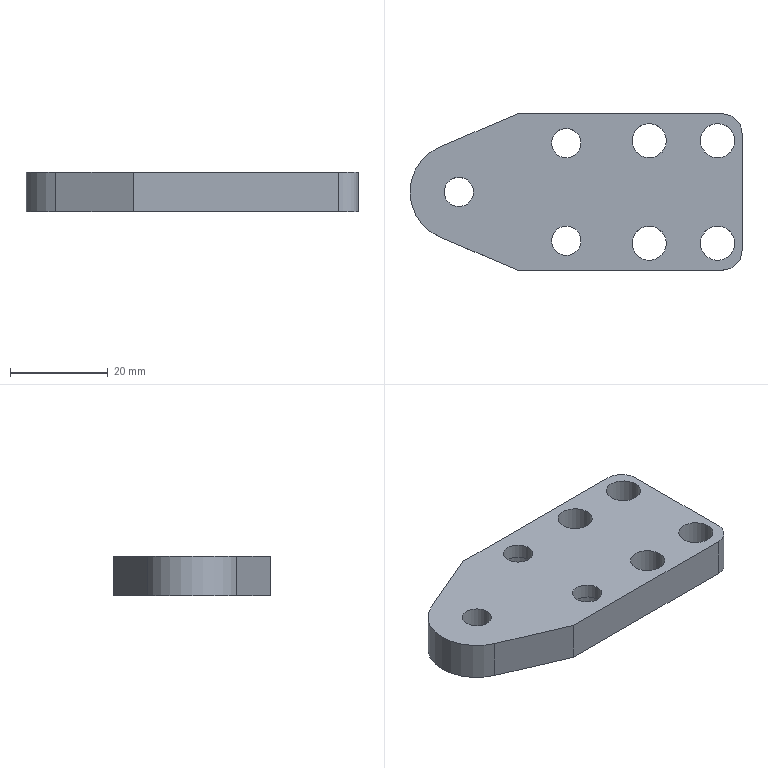Part | NX | features BREP 1, DATUM_CSYS 1 | 1 solid | 21 faces | box 68 x 32 x 8 mm | volume 13164 mm3 | cylinder 12 | plane 9 | commonest cylinder face diameters 7 x4 6 x3 8 x2 10 x2 20 x1
STEP:
#1=CARTESIAN_POINT('',(-34.,16.,0.));
#2=VERTEX_POINT('',#1);
#3=CARTESIAN_POINT('',(-49.928,9.196,0.));
#4=VERTEX_POINT('',#3);
#5=CARTESIAN_POINT('',(-34.,16.,0.));
#6=DIRECTION('',(-0.9196,-0.3928,0.));
#7=VECTOR('',#6,1000.);
#8=LINE('',#5,#7);
#9=EDGE_CURVE('',#2,#4,#8,.T.);
#10=ORIENTED_EDGE('',*,*,#9,.T.);
#11=CARTESIAN_POINT('',(-49.928,9.196,8.));
#12=VERTEX_POINT('',#11);
#13=CARTESIAN_POINT('',(-49.928,9.196,0.));
#14=DIRECTION('',(0.,0.,1.));
#15=VECTOR('',#14,1000.);
#16=LINE('',#13,#15);
#17=EDGE_CURVE('',#4,#12,#16,.T.);
#18=ORIENTED_EDGE('',*,*,#17,.T.);
#19=CARTESIAN_POINT('',(-34.,16.,8.));
#20=VERTEX_POINT('',#19);
#21=CARTESIAN_POINT('',(-34.,16.,8.));
#22=DIRECTION('',(-0.9196,-0.3928,0.));
#23=VECTOR('',#22,1000.);
#24=LINE('',#21,#23);
#25=EDGE_CURVE('',#20,#12,#24,.T.);
#26=ORIENTED_EDGE('',*,*,#25,.F.);
#27=CARTESIAN_POINT('',(-34.,16.,0.));
#28=DIRECTION('',(0.,0.,1.));
#29=VECTOR('',#28,1000.);
#30=LINE('',#27,#29);
#31=EDGE_CURVE('',#2,#20,#30,.T.);
#32=ORIENTED_EDGE('',*,*,#31,.F.);
#33=EDGE_LOOP('',(#10,#18,#26,#32));
#34=FACE_BOUND('',#33,.T.);
#35=CARTESIAN_POINT('',(-41.964,12.598,4.));
#36=DIRECTION('',(-0.3928,0.9196,0.));
#37=DIRECTION('',(0.9196,0.3928,0.));
#38=AXIS2_PLACEMENT_3D('',#35,#36,#37);
#39=PLANE('',#38);
#40=ADVANCED_FACE('',(#34),#39,.T.);
#41=CARTESIAN_POINT('',(-49.928,-9.196,0.));
#42=VERTEX_POINT('',#41);
#43=CARTESIAN_POINT('',(-46.,0.,0.));
#44=DIRECTION('',(0.,0.,1.));
#45=DIRECTION('',(-0.3928,0.9196,0.));
#46=AXIS2_PLACEMENT_3D('',#43,#44,#45);
#47=CIRCLE('',#46,10.);
#48=EDGE_CURVE('',#4,#42,#47,.T.);
#49=ORIENTED_EDGE('',*,*,#48,.T.);
#50=CARTESIAN_POINT('',(-49.928,-9.196,8.));
#51=VERTEX_POINT('',#50);
#52=CARTESIAN_POINT('',(-49.928,-9.196,0.));
#53=DIRECTION('',(0.,0.,1.));
#54=VECTOR('',#53,1000.);
#55=LINE('',#52,#54);
#56=EDGE_CURVE('',#42,#51,#55,.T.);
#57=ORIENTED_EDGE('',*,*,#56,.T.);
#58=CARTESIAN_POINT('',(-46.,0.,8.));
#59=DIRECTION('',(0.,0.,1.));
#60=DIRECTION('',(-0.3928,0.9196,0.));
#61=AXIS2_PLACEMENT_3D('',#58,#59,#60);
#62=CIRCLE('',#61,10.);
#63=EDGE_CURVE('',#12,#51,#62,.T.);
#64=ORIENTED_EDGE('',*,*,#63,.F.);
#65=ORIENTED_EDGE('',*,*,#17,.F.);
#66=EDGE_LOOP('',(#49,#57,#64,#65));
#67=FACE_BOUND('',#66,.T.);
#68=CARTESIAN_POINT('',(-46.,0.,0.));
#69=DIRECTION('',(0.,0.,1.));
#70=DIRECTION('',(0.3928,-0.9196,0.));
#71=AXIS2_PLACEMENT_3D('',#68,#69,#70);
#72=CYLINDRICAL_SURFACE('',#71,10.);
#73=ADVANCED_FACE('',(#67),#72,.T.);
#74=CARTESIAN_POINT('',(-34.,-16.,0.));
#75=VERTEX_POINT('',#74);
#76=CARTESIAN_POINT('',(-49.928,-9.196,0.));
#77=DIRECTION('',(0.9196,-0.3928,0.));
#78=VECTOR('',#77,1000.);
#79=LINE('',#76,#78);
#80=EDGE_CURVE('',#42,#75,#79,.T.);
#81=ORIENTED_EDGE('',*,*,#80,.T.);
#82=CARTESIAN_POINT('',(-34.,-16.,8.));
#83=VERTEX_POINT('',#82);
#84=CARTESIAN_POINT('',(-34.,-16.,0.));
#85=DIRECTION('',(0.,0.,1.));
#86=VECTOR('',#85,1000.);
#87=LINE('',#84,#86);
#88=EDGE_CURVE('',#75,#83,#87,.T.);
#89=ORIENTED_EDGE('',*,*,#88,.T.);
#90=CARTESIAN_POINT('',(-49.928,-9.196,8.));
#91=DIRECTION('',(0.9196,-0.3928,0.));
#92=VECTOR('',#91,1000.);
#93=LINE('',#90,#92);
#94=EDGE_CURVE('',#51,#83,#93,.T.);
#95=ORIENTED_EDGE('',*,*,#94,.F.);
#96=ORIENTED_EDGE('',*,*,#56,.F.);
#97=EDGE_LOOP('',(#81,#89,#95,#96));
#98=FACE_BOUND('',#97,.T.);
#99=CARTESIAN_POINT('',(-41.964,-12.598,4.));
#100=DIRECTION('',(-0.3928,-0.9196,0.));
#101=DIRECTION('',(-0.9196,0.3928,0.));
#102=AXIS2_PLACEMENT_3D('',#99,#100,#101);
#103=PLANE('',#102);
#104=ADVANCED_FACE('',(#98),#103,.T.);
#105=CARTESIAN_POINT('',(12.,-12.,0.));
#106=VERTEX_POINT('',#105);
#107=CARTESIAN_POINT('',(12.,12.,0.));
#108=VERTEX_POINT('',#107);
#109=CARTESIAN_POINT('',(12.,-12.,0.));
#110=DIRECTION('',(0.,1.,0.));
#111=VECTOR('',#110,1000.);
#112=LINE('',#109,#111);
#113=EDGE_CURVE('',#106,#108,#112,.T.);
#114=ORIENTED_EDGE('',*,*,#113,.T.);
#115=CARTESIAN_POINT('',(12.,12.,8.));
#116=VERTEX_POINT('',#115);
#117=CARTESIAN_POINT('',(12.,12.,0.));
#118=DIRECTION('',(0.,0.,1.));
#119=VECTOR('',#118,1000.);
#120=LINE('',#117,#119);
#121=EDGE_CURVE('',#108,#116,#120,.T.);
#122=ORIENTED_EDGE('',*,*,#121,.T.);
#123=CARTESIAN_POINT('',(12.,-12.,8.));
#124=VERTEX_POINT('',#123);
#125=CARTESIAN_POINT('',(12.,-12.,8.));
#126=DIRECTION('',(0.,1.,0.));
#127=VECTOR('',#126,1000.);
#128=LINE('',#125,#127);
#129=EDGE_CURVE('',#124,#116,#128,.T.);
#130=ORIENTED_EDGE('',*,*,#129,.F.);
#131=CARTESIAN_POINT('',(12.,-12.,0.));
#132=DIRECTION('',(0.,0.,1.));
#133=VECTOR('',#132,1000.);
#134=LINE('',#131,#133);
#135=EDGE_CURVE('',#106,#124,#134,.T.);
#136=ORIENTED_EDGE('',*,*,#135,.F.);
#137=EDGE_LOOP('',(#114,#122,#130,#136));
#138=FACE_BOUND('',#137,.T.);
#139=CARTESIAN_POINT('',(12.,0.,4.));
#140=DIRECTION('',(1.,0.,0.));
#141=DIRECTION('',(0.,-1.,0.));
#142=AXIS2_PLACEMENT_3D('',#139,#140,#141);
#143=PLANE('',#142);
#144=ADVANCED_FACE('',(#138),#143,.T.);
#145=CARTESIAN_POINT('',(8.,16.,8.));
#146=VERTEX_POINT('',#145);
#147=CARTESIAN_POINT('',(8.,16.,8.));
#148=DIRECTION('',(-1.,0.,0.));
#149=VECTOR('',#148,1000.);
#150=LINE('',#147,#149);
#151=EDGE_CURVE('',#146,#20,#150,.T.);
#152=ORIENTED_EDGE('',*,*,#151,.F.);
#153=CARTESIAN_POINT('',(8.,16.,0.));
#154=VERTEX_POINT('',#153);
#155=CARTESIAN_POINT('',(8.,16.,0.));
#156=DIRECTION('',(0.,0.,1.));
#157=VECTOR('',#156,1000.);
#158=LINE('',#155,#157);
#159=EDGE_CURVE('',#154,#146,#158,.T.);
#160=ORIENTED_EDGE('',*,*,#159,.F.);
#161=CARTESIAN_POINT('',(8.,16.,0.));
#162=DIRECTION('',(-1.,0.,0.));
#163=VECTOR('',#162,1000.);
#164=LINE('',#161,#163);
#165=EDGE_CURVE('',#154,#2,#164,.T.);
#166=ORIENTED_EDGE('',*,*,#165,.T.);
#167=ORIENTED_EDGE('',*,*,#31,.T.);
#168=EDGE_LOOP('',(#152,#160,#166,#167));
#169=FACE_BOUND('',#168,.T.);
#170=CARTESIAN_POINT('',(-11.,16.,4.));
#171=DIRECTION('',(0.,1.,0.));
#172=DIRECTION('',(1.,0.,0.));
#173=AXIS2_PLACEMENT_3D('',#170,#171,#172);
#174=PLANE('',#173);
#175=ADVANCED_FACE('',(#169),#174,.T.);
#176=CARTESIAN_POINT('',(8.,-16.,0.));
#177=VERTEX_POINT('',#176);
#178=CARTESIAN_POINT('',(-34.,-16.,0.));
#179=DIRECTION('',(1.,0.,0.));
#180=VECTOR('',#179,1000.);
#181=LINE('',#178,#180);
#182=EDGE_CURVE('',#75,#177,#181,.T.);
#183=ORIENTED_EDGE('',*,*,#182,.T.);
#184=CARTESIAN_POINT('',(8.,-16.,8.));
#185=VERTEX_POINT('',#184);
#186=CARTESIAN_POINT('',(8.,-16.,0.));
#187=DIRECTION('',(0.,0.,1.));
#188=VECTOR('',#187,1000.);
#189=LINE('',#186,#188);
#190=EDGE_CURVE('',#177,#185,#189,.T.);
#191=ORIENTED_EDGE('',*,*,#190,.T.);
#192=CARTESIAN_POINT('',(-34.,-16.,8.));
#193=DIRECTION('',(1.,0.,0.));
#194=VECTOR('',#193,1000.);
#195=LINE('',#192,#194);
#196=EDGE_CURVE('',#83,#185,#195,.T.);
#197=ORIENTED_EDGE('',*,*,#196,.F.);
#198=ORIENTED_EDGE('',*,*,#88,.F.);
#199=EDGE_LOOP('',(#183,#191,#197,#198));
#200=FACE_BOUND('',#199,.T.);
#201=CARTESIAN_POINT('',(-11.,-16.,4.));
#202=DIRECTION('',(0.,-1.,0.));
#203=DIRECTION('',(-1.,0.,0.));
#204=AXIS2_PLACEMENT_3D('',#201,#202,#203);
#205=PLANE('',#204);
#206=ADVANCED_FACE('',(#200),#205,.T.);
#207=CARTESIAN_POINT('',(8.,-12.,0.));
#208=DIRECTION('',(0.,0.,1.));
#209=DIRECTION('',(0.,-1.,0.));
#210=AXIS2_PLACEMENT_3D('',#207,#208,#209);
#211=CIRCLE('',#210,4.);
#212=EDGE_CURVE('',#177,#106,#211,.T.);
#213=ORIENTED_EDGE('',*,*,#212,.T.);
#214=ORIENTED_EDGE('',*,*,#135,.T.);
#215=CARTESIAN_POINT('',(8.,-12.,8.));
#216=DIRECTION('',(0.,0.,1.));
#217=DIRECTION('',(0.,-1.,0.));
#218=AXIS2_PLACEMENT_3D('',#215,#216,#217);
#219=CIRCLE('',#218,4.);
#220=EDGE_CURVE('',#185,#124,#219,.T.);
#221=ORIENTED_EDGE('',*,*,#220,.F.);
#222=ORIENTED_EDGE('',*,*,#190,.F.);
#223=EDGE_LOOP('',(#213,#214,#221,#222));
#224=FACE_BOUND('',#223,.T.);
#225=CARTESIAN_POINT('',(8.,-12.,0.));
#226=DIRECTION('',(0.,0.,1.));
#227=DIRECTION('',(0.,1.,0.));
#228=AXIS2_PLACEMENT_3D('',#225,#226,#227);
#229=CYLINDRICAL_SURFACE('',#228,4.);
#230=ADVANCED_FACE('',(#224),#229,.T.);
#231=CARTESIAN_POINT('',(8.,12.,0.));
#232=DIRECTION('',(0.,0.,1.));
#233=DIRECTION('',(1.,0.,0.));
#234=AXIS2_PLACEMENT_3D('',#231,#232,#233);
#235=CIRCLE('',#234,4.);
#236=EDGE_CURVE('',#108,#154,#235,.T.);
#237=ORIENTED_EDGE('',*,*,#236,.T.);
#238=ORIENTED_EDGE('',*,*,#159,.T.);
#239=CARTESIAN_POINT('',(8.,12.,8.));
#240=DIRECTION('',(0.,0.,1.));
#241=DIRECTION('',(1.,0.,0.));
#242=AXIS2_PLACEMENT_3D('',#239,#240,#241);
#243=CIRCLE('',#242,4.);
#244=EDGE_CURVE('',#116,#146,#243,.T.);
#245=ORIENTED_EDGE('',*,*,#244,.F.);
#246=ORIENTED_EDGE('',*,*,#121,.F.);
#247=EDGE_LOOP('',(#237,#238,#245,#246));
#248=FACE_BOUND('',#247,.T.);
#249=CARTESIAN_POINT('',(8.,12.,0.));
#250=DIRECTION('',(0.,0.,1.));
#251=DIRECTION('',(-1.,0.,0.));
#252=AXIS2_PLACEMENT_3D('',#249,#250,#251);
#253=CYLINDRICAL_SURFACE('',#252,4.);
#254=ADVANCED_FACE('',(#248),#253,.T.);
#255=CARTESIAN_POINT('',(-3.5,10.5,8.));
#256=VERTEX_POINT('',#255);
#257=CARTESIAN_POINT('',(-3.5,10.5,0.));
#258=VERTEX_POINT('',#257);
#259=CARTESIAN_POINT('',(-3.5,10.5,8.));
#260=DIRECTION('',(0.,0.,-1.));
#261=VECTOR('',#260,1000.);
#262=LINE('',#259,#261);
#263=EDGE_CURVE('',#256,#258,#262,.T.);
#264=ORIENTED_EDGE('',*,*,#263,.T.);
#265=CARTESIAN_POINT('',(-7.,10.5,0.));
#266=DIRECTION('',(0.,0.,-1.));
#267=DIRECTION('',(1.,0.,0.));
#268=AXIS2_PLACEMENT_3D('',#265,#266,#267);
#269=CIRCLE('',#268,3.5);
#270=EDGE_CURVE('',#258,#258,#269,.T.);
#271=ORIENTED_EDGE('',*,*,#270,.T.);
#272=ORIENTED_EDGE('',*,*,#263,.F.);
#273=CARTESIAN_POINT('',(-7.,10.5,8.));
#274=DIRECTION('',(0.,0.,-1.));
#275=DIRECTION('',(1.,0.,0.));
#276=AXIS2_PLACEMENT_3D('',#273,#274,#275);
#277=CIRCLE('',#276,3.5);
#278=EDGE_CURVE('',#256,#256,#277,.T.);
#279=ORIENTED_EDGE('',*,*,#278,.F.);
#280=EDGE_LOOP('',(#264,#271,#272,#279));
#281=FACE_BOUND('',#280,.T.);
#282=CARTESIAN_POINT('',(-7.,10.5,8.));
#283=DIRECTION('',(0.,0.,-1.));
#284=DIRECTION('',(-1.,0.,0.));
#285=AXIS2_PLACEMENT_3D('',#282,#283,#284);
#286=CYLINDRICAL_SURFACE('',#285,3.5);
#287=ADVANCED_FACE('',(#281),#286,.F.);
#288=CARTESIAN_POINT('',(10.5,10.5,8.));
#289=VERTEX_POINT('',#288);
#290=CARTESIAN_POINT('',(10.5,10.5,0.));
#291=VERTEX_POINT('',#290);
#292=CARTESIAN_POINT('',(10.5,10.5,8.));
#293=DIRECTION('',(0.,0.,-1.));
#294=VECTOR('',#293,1000.);
#295=LINE('',#292,#294);
#296=EDGE_CURVE('',#289,#291,#295,.T.);
#297=ORIENTED_EDGE('',*,*,#296,.T.);
#298=CARTESIAN_POINT('',(7.,10.5,0.));
#299=DIRECTION('',(0.,0.,-1.));
#300=DIRECTION('',(1.,0.,0.));
#301=AXIS2_PLACEMENT_3D('',#298,#299,#300);
#302=CIRCLE('',#301,3.5);
#303=EDGE_CURVE('',#291,#291,#302,.T.);
#304=ORIENTED_EDGE('',*,*,#303,.T.);
#305=ORIENTED_EDGE('',*,*,#296,.F.);
#306=CARTESIAN_POINT('',(7.,10.5,8.));
#307=DIRECTION('',(0.,0.,-1.));
#308=DIRECTION('',(1.,0.,0.));
#309=AXIS2_PLACEMENT_3D('',#306,#307,#308);
#310=CIRCLE('',#309,3.5);
#311=EDGE_CURVE('',#289,#289,#310,.T.);
#312=ORIENTED_EDGE('',*,*,#311,.F.);
#313=EDGE_LOOP('',(#297,#304,#305,#312));
#314=FACE_BOUND('',#313,.T.);
#315=CARTESIAN_POINT('',(7.,10.5,8.));
#316=DIRECTION('',(0.,0.,-1.));
#317=DIRECTION('',(-1.,0.,0.));
#318=AXIS2_PLACEMENT_3D('',#315,#316,#317);
#319=CYLINDRICAL_SURFACE('',#318,3.5);
#320=ADVANCED_FACE('',(#314),#319,.F.);
#321=CARTESIAN_POINT('',(-3.5,-10.5,8.));
#322=VERTEX_POINT('',#321);
#323=CARTESIAN_POINT('',(-3.5,-10.5,0.));
#324=VERTEX_POINT('',#323);
#325=CARTESIAN_POINT('',(-3.5,-10.5,8.));
#326=DIRECTION('',(0.,0.,-1.));
#327=VECTOR('',#326,1000.);
#328=LINE('',#325,#327);
#329=EDGE_CURVE('',#322,#324,#328,.T.);
#330=ORIENTED_EDGE('',*,*,#329,.T.);
#331=CARTESIAN_POINT('',(-7.,-10.5,0.));
#332=DIRECTION('',(0.,0.,-1.));
#333=DIRECTION('',(1.,0.,0.));
#334=AXIS2_PLACEMENT_3D('',#331,#332,#333);
#335=CIRCLE('',#334,3.5);
#336=EDGE_CURVE('',#324,#324,#335,.T.);
#337=ORIENTED_EDGE('',*,*,#336,.T.);
#338=ORIENTED_EDGE('',*,*,#329,.F.);
#339=CARTESIAN_POINT('',(-7.,-10.5,8.));
#340=DIRECTION('',(0.,0.,-1.));
#341=DIRECTION('',(1.,0.,0.));
#342=AXIS2_PLACEMENT_3D('',#339,#340,#341);
#343=CIRCLE('',#342,3.5);
#344=EDGE_CURVE('',#322,#322,#343,.T.);
#345=ORIENTED_EDGE('',*,*,#344,.F.);
#346=EDGE_LOOP('',(#330,#337,#338,#345));
#347=FACE_BOUND('',#346,.T.);
#348=CARTESIAN_POINT('',(-7.,-10.5,8.));
#349=DIRECTION('',(0.,0.,-1.));
#350=DIRECTION('',(-1.,0.,0.));
#351=AXIS2_PLACEMENT_3D('',#348,#349,#350);
#352=CYLINDRICAL_SURFACE('',#351,3.5);
#353=ADVANCED_FACE('',(#347),#352,.F.);
#354=CARTESIAN_POINT('',(10.5,-10.5,8.));
#355=VERTEX_POINT('',#354);
#356=CARTESIAN_POINT('',(10.5,-10.5,0.));
#357=VERTEX_POINT('',#356);
#358=CARTESIAN_POINT('',(10.5,-10.5,8.));
#359=DIRECTION('',(0.,0.,-1.));
#360=VECTOR('',#359,1000.);
#361=LINE('',#358,#360);
#362=EDGE_CURVE('',#355,#357,#361,.T.);
#363=ORIENTED_EDGE('',*,*,#362,.T.);
#364=CARTESIAN_POINT('',(7.,-10.5,0.));
#365=DIRECTION('',(0.,0.,-1.));
#366=DIRECTION('',(1.,0.,0.));
#367=AXIS2_PLACEMENT_3D('',#364,#365,#366);
#368=CIRCLE('',#367,3.5);
#369=EDGE_CURVE('',#357,#357,#368,.T.);
#370=ORIENTED_EDGE('',*,*,#369,.T.);
#371=ORIENTED_EDGE('',*,*,#362,.F.);
#372=CARTESIAN_POINT('',(7.,-10.5,8.));
#373=DIRECTION('',(0.,0.,-1.));
#374=DIRECTION('',(1.,0.,0.));
#375=AXIS2_PLACEMENT_3D('',#372,#373,#374);
#376=CIRCLE('',#375,3.5);
#377=EDGE_CURVE('',#355,#355,#376,.T.);
#378=ORIENTED_EDGE('',*,*,#377,.F.);
#379=EDGE_LOOP('',(#363,#370,#371,#378));
#380=FACE_BOUND('',#379,.T.);
#381=CARTESIAN_POINT('',(7.,-10.5,8.));
#382=DIRECTION('',(0.,0.,-1.));
#383=DIRECTION('',(-1.,0.,0.));
#384=AXIS2_PLACEMENT_3D('',#381,#382,#383);
#385=CYLINDRICAL_SURFACE('',#384,3.5);
#386=ADVANCED_FACE('',(#380),#385,.F.);
#387=ORIENTED_EDGE('',*,*,#165,.F.);
#388=ORIENTED_EDGE('',*,*,#236,.F.);
#389=ORIENTED_EDGE('',*,*,#113,.F.);
#390=ORIENTED_EDGE('',*,*,#212,.F.);
#391=ORIENTED_EDGE('',*,*,#182,.F.);
#392=ORIENTED_EDGE('',*,*,#80,.F.);
#393=ORIENTED_EDGE('',*,*,#48,.F.);
#394=ORIENTED_EDGE('',*,*,#9,.F.);
#395=EDGE_LOOP('',(#387,#388,#389,#390,#391,#392,#393,#394));
#396=FACE_BOUND('',#395,.T.);
#397=CARTESIAN_POINT('',(-19.,10.,0.));
#398=VERTEX_POINT('',#397);
#399=CARTESIAN_POINT('',(-24.,10.,0.));
#400=DIRECTION('',(0.,0.,1.));
#401=DIRECTION('',(1.,0.,0.));
#402=AXIS2_PLACEMENT_3D('',#399,#400,#401);
#403=CIRCLE('',#402,5.);
#404=EDGE_CURVE('',#398,#398,#403,.T.);
#405=ORIENTED_EDGE('',*,*,#404,.T.);
#406=EDGE_LOOP('',(#405));
#407=FACE_BOUND('',#406,.T.);
#408=ORIENTED_EDGE('',*,*,#270,.F.);
#409=EDGE_LOOP('',(#408));
#410=FACE_BOUND('',#409,.T.);
#411=ORIENTED_EDGE('',*,*,#303,.F.);
#412=EDGE_LOOP('',(#411));
#413=FACE_BOUND('',#412,.T.);
#414=ORIENTED_EDGE('',*,*,#336,.F.);
#415=EDGE_LOOP('',(#414));
#416=FACE_BOUND('',#415,.T.);
#417=ORIENTED_EDGE('',*,*,#369,.F.);
#418=EDGE_LOOP('',(#417));
#419=FACE_BOUND('',#418,.T.);
#420=CARTESIAN_POINT('',(-19.,-10.,0.));
#421=VERTEX_POINT('',#420);
#422=CARTESIAN_POINT('',(-24.,-10.,0.));
#423=DIRECTION('',(0.,0.,1.));
#424=DIRECTION('',(1.,0.,0.));
#425=AXIS2_PLACEMENT_3D('',#422,#423,#424);
#426=CIRCLE('',#425,5.);
#427=EDGE_CURVE('',#421,#421,#426,.T.);
#428=ORIENTED_EDGE('',*,*,#427,.T.);
#429=EDGE_LOOP('',(#428));
#430=FACE_BOUND('',#429,.T.);
#431=CARTESIAN_POINT('',(-43.,0.,0.));
#432=VERTEX_POINT('',#431);
#433=CARTESIAN_POINT('',(-46.,0.,0.));
#434=DIRECTION('',(0.,0.,-1.));
#435=DIRECTION('',(1.,0.,0.));
#436=AXIS2_PLACEMENT_3D('',#433,#434,#435);
#437=CIRCLE('',#436,3.);
#438=EDGE_CURVE('',#432,#432,#437,.T.);
#439=ORIENTED_EDGE('',*,*,#438,.F.);
#440=EDGE_LOOP('',(#439));
#441=FACE_BOUND('',#440,.T.);
#442=CARTESIAN_POINT('',(-22.,18.,0.));
#443=DIRECTION('',(0.,0.,1.));
#444=DIRECTION('',(-1.,0.,0.));
#445=AXIS2_PLACEMENT_3D('',#442,#443,#444);
#446=PLANE('',#445);
#447=ADVANCED_FACE('',(#396,#407,#410,#413,#416,#419,#430,#441),#446,.F.);
#448=ORIENTED_EDGE('',*,*,#25,.T.);
#449=ORIENTED_EDGE('',*,*,#63,.T.);
#450=ORIENTED_EDGE('',*,*,#94,.T.);
#451=ORIENTED_EDGE('',*,*,#196,.T.);
#452=ORIENTED_EDGE('',*,*,#220,.T.);
#453=ORIENTED_EDGE('',*,*,#129,.T.);
#454=ORIENTED_EDGE('',*,*,#244,.T.);
#455=ORIENTED_EDGE('',*,*,#151,.T.);
#456=EDGE_LOOP('',(#448,#449,#450,#451,#452,#453,#454,#455));
#457=FACE_BOUND('',#456,.T.);
#458=CARTESIAN_POINT('',(-21.,10.,8.));
#459=VERTEX_POINT('',#458);
#460=CARTESIAN_POINT('',(-24.,10.,8.));
#461=DIRECTION('',(0.,0.,-1.));
#462=DIRECTION('',(1.,0.,0.));
#463=AXIS2_PLACEMENT_3D('',#460,#461,#462);
#464=CIRCLE('',#463,3.);
#465=EDGE_CURVE('',#459,#459,#464,.T.);
#466=ORIENTED_EDGE('',*,*,#465,.T.);
#467=EDGE_LOOP('',(#466));
#468=FACE_BOUND('',#467,.T.);
#469=CARTESIAN_POINT('',(-21.,-10.,8.));
#470=VERTEX_POINT('',#469);
#471=CARTESIAN_POINT('',(-24.,-10.,8.));
#472=DIRECTION('',(0.,0.,-1.));
#473=DIRECTION('',(1.,0.,0.));
#474=AXIS2_PLACEMENT_3D('',#471,#472,#473);
#475=CIRCLE('',#474,3.);
#476=EDGE_CURVE('',#470,#470,#475,.T.);
#477=ORIENTED_EDGE('',*,*,#476,.T.);
#478=EDGE_LOOP('',(#477));
#479=FACE_BOUND('',#478,.T.);
#480=ORIENTED_EDGE('',*,*,#278,.T.);
#481=EDGE_LOOP('',(#480));
#482=FACE_BOUND('',#481,.T.);
#483=ORIENTED_EDGE('',*,*,#311,.T.);
#484=EDGE_LOOP('',(#483));
#485=FACE_BOUND('',#484,.T.);
#486=ORIENTED_EDGE('',*,*,#344,.T.);
#487=EDGE_LOOP('',(#486));
#488=FACE_BOUND('',#487,.T.);
#489=ORIENTED_EDGE('',*,*,#377,.T.);
#490=EDGE_LOOP('',(#489));
#491=FACE_BOUND('',#490,.T.);
#492=CARTESIAN_POINT('',(-43.,0.,8.));
#493=VERTEX_POINT('',#492);
#494=CARTESIAN_POINT('',(-46.,0.,8.));
#495=DIRECTION('',(0.,0.,-1.));
#496=DIRECTION('',(1.,0.,0.));
#497=AXIS2_PLACEMENT_3D('',#494,#495,#496);
#498=CIRCLE('',#497,3.);
#499=EDGE_CURVE('',#493,#493,#498,.T.);
#500=ORIENTED_EDGE('',*,*,#499,.T.);
#501=EDGE_LOOP('',(#500));
#502=FACE_BOUND('',#501,.T.);
#503=CARTESIAN_POINT('',(-22.,18.,8.));
#504=DIRECTION('',(0.,0.,1.));
#505=DIRECTION('',(-1.,0.,0.));
#506=AXIS2_PLACEMENT_3D('',#503,#504,#505);
#507=PLANE('',#506);
#508=ADVANCED_FACE('',(#457,#468,#479,#482,#485,#488,#491,#502),#507,.T.);
#509=CARTESIAN_POINT('',(-21.,-10.,5.));
#510=VERTEX_POINT('',#509);
#511=CARTESIAN_POINT('',(-21.,-10.,8.));
#512=DIRECTION('',(0.,0.,-1.));
#513=VECTOR('',#512,1000.);
#514=LINE('',#511,#513);
#515=EDGE_CURVE('',#470,#510,#514,.T.);
#516=ORIENTED_EDGE('',*,*,#515,.T.);
#517=CARTESIAN_POINT('',(-24.,-10.,5.));
#518=DIRECTION('',(0.,0.,1.));
#519=DIRECTION('',(1.,0.,0.));
#520=AXIS2_PLACEMENT_3D('',#517,#518,#519);
#521=CIRCLE('',#520,3.);
#522=EDGE_CURVE('',#510,#510,#521,.T.);
#523=ORIENTED_EDGE('',*,*,#522,.F.);
#524=ORIENTED_EDGE('',*,*,#515,.F.);
#525=ORIENTED_EDGE('',*,*,#476,.F.);
#526=EDGE_LOOP('',(#516,#523,#524,#525));
#527=FACE_BOUND('',#526,.T.);
#528=CARTESIAN_POINT('',(-24.,-10.,8.));
#529=DIRECTION('',(0.,0.,-1.));
#530=DIRECTION('',(-1.,0.,0.));
#531=AXIS2_PLACEMENT_3D('',#528,#529,#530);
#532=CYLINDRICAL_SURFACE('',#531,3.);
#533=ADVANCED_FACE('',(#527),#532,.F.);
#534=CARTESIAN_POINT('',(-21.,10.,5.));
#535=VERTEX_POINT('',#534);
#536=CARTESIAN_POINT('',(-21.,10.,8.));
#537=DIRECTION('',(0.,0.,-1.));
#538=VECTOR('',#537,1000.);
#539=LINE('',#536,#538);
#540=EDGE_CURVE('',#459,#535,#539,.T.);
#541=ORIENTED_EDGE('',*,*,#540,.T.);
#542=CARTESIAN_POINT('',(-24.,10.,5.));
#543=DIRECTION('',(0.,0.,1.));
#544=DIRECTION('',(1.,0.,0.));
#545=AXIS2_PLACEMENT_3D('',#542,#543,#544);
#546=CIRCLE('',#545,3.);
#547=EDGE_CURVE('',#535,#535,#546,.T.);
#548=ORIENTED_EDGE('',*,*,#547,.F.);
#549=ORIENTED_EDGE('',*,*,#540,.F.);
#550=ORIENTED_EDGE('',*,*,#465,.F.);
#551=EDGE_LOOP('',(#541,#548,#549,#550));
#552=FACE_BOUND('',#551,.T.);
#553=CARTESIAN_POINT('',(-24.,10.,8.));
#554=DIRECTION('',(0.,0.,-1.));
#555=DIRECTION('',(-1.,0.,0.));
#556=AXIS2_PLACEMENT_3D('',#553,#554,#555);
#557=CYLINDRICAL_SURFACE('',#556,3.);
#558=ADVANCED_FACE('',(#552),#557,.F.);
#559=CARTESIAN_POINT('',(-19.,-10.,5.));
#560=VERTEX_POINT('',#559);
#561=CARTESIAN_POINT('',(-19.,-10.,0.));
#562=DIRECTION('',(0.,0.,1.));
#563=VECTOR('',#562,1000.);
#564=LINE('',#561,#563);
#565=EDGE_CURVE('',#421,#560,#564,.T.);
#566=ORIENTED_EDGE('',*,*,#565,.T.);
#567=CARTESIAN_POINT('',(-24.,-10.,5.));
#568=DIRECTION('',(0.,0.,1.));
#569=DIRECTION('',(1.,0.,0.));
#570=AXIS2_PLACEMENT_3D('',#567,#568,#569);
#571=CIRCLE('',#570,5.);
#572=EDGE_CURVE('',#560,#560,#571,.T.);
#573=ORIENTED_EDGE('',*,*,#572,.T.);
#574=ORIENTED_EDGE('',*,*,#565,.F.);
#575=ORIENTED_EDGE('',*,*,#427,.F.);
#576=EDGE_LOOP('',(#566,#573,#574,#575));
#577=FACE_BOUND('',#576,.T.);
#578=CARTESIAN_POINT('',(-24.,-10.,0.));
#579=DIRECTION('',(0.,0.,1.));
#580=DIRECTION('',(-1.,0.,0.));
#581=AXIS2_PLACEMENT_3D('',#578,#579,#580);
#582=CYLINDRICAL_SURFACE('',#581,5.);
#583=ADVANCED_FACE('',(#577),#582,.F.);
#584=ORIENTED_EDGE('',*,*,#572,.F.);
#585=EDGE_LOOP('',(#584));
#586=FACE_BOUND('',#585,.T.);
#587=ORIENTED_EDGE('',*,*,#522,.T.);
#588=EDGE_LOOP('',(#587));
#589=FACE_BOUND('',#588,.T.);
#590=CARTESIAN_POINT('',(-24.,-10.,5.));
#591=DIRECTION('',(0.,0.,1.));
#592=DIRECTION('',(-1.,0.,0.));
#593=AXIS2_PLACEMENT_3D('',#590,#591,#592);
#594=PLANE('',#593);
#595=ADVANCED_FACE('',(#586,#589),#594,.F.);
#596=CARTESIAN_POINT('',(-19.,10.,5.));
#597=VERTEX_POINT('',#596);
#598=CARTESIAN_POINT('',(-19.,10.,0.));
#599=DIRECTION('',(0.,0.,1.));
#600=VECTOR('',#599,1000.);
#601=LINE('',#598,#600);
#602=EDGE_CURVE('',#398,#597,#601,.T.);
#603=ORIENTED_EDGE('',*,*,#602,.T.);
#604=CARTESIAN_POINT('',(-24.,10.,5.));
#605=DIRECTION('',(0.,0.,1.));
#606=DIRECTION('',(1.,0.,0.));
#607=AXIS2_PLACEMENT_3D('',#604,#605,#606);
#608=CIRCLE('',#607,5.);
#609=EDGE_CURVE('',#597,#597,#608,.T.);
#610=ORIENTED_EDGE('',*,*,#609,.T.);
#611=ORIENTED_EDGE('',*,*,#602,.F.);
#612=ORIENTED_EDGE('',*,*,#404,.F.);
#613=EDGE_LOOP('',(#603,#610,#611,#612));
#614=FACE_BOUND('',#613,.T.);
#615=CARTESIAN_POINT('',(-24.,10.,0.));
#616=DIRECTION('',(0.,0.,1.));
#617=DIRECTION('',(-1.,0.,0.));
#618=AXIS2_PLACEMENT_3D('',#615,#616,#617);
#619=CYLINDRICAL_SURFACE('',#618,5.);
#620=ADVANCED_FACE('',(#614),#619,.F.);
#621=ORIENTED_EDGE('',*,*,#609,.F.);
#622=EDGE_LOOP('',(#621));
#623=FACE_BOUND('',#622,.T.);
#624=ORIENTED_EDGE('',*,*,#547,.T.);
#625=EDGE_LOOP('',(#624));
#626=FACE_BOUND('',#625,.T.);
#627=CARTESIAN_POINT('',(-24.,10.,5.));
#628=DIRECTION('',(0.,0.,1.));
#629=DIRECTION('',(-1.,0.,0.));
#630=AXIS2_PLACEMENT_3D('',#627,#628,#629);
#631=PLANE('',#630);
#632=ADVANCED_FACE('',(#623,#626),#631,.F.);
#633=CARTESIAN_POINT('',(-43.,0.,8.));
#634=DIRECTION('',(0.,0.,-1.));
#635=VECTOR('',#634,1000.);
#636=LINE('',#633,#635);
#637=EDGE_CURVE('',#493,#432,#636,.T.);
#638=ORIENTED_EDGE('',*,*,#637,.T.);
#639=ORIENTED_EDGE('',*,*,#438,.T.);
#640=ORIENTED_EDGE('',*,*,#637,.F.);
#641=ORIENTED_EDGE('',*,*,#499,.F.);
#642=EDGE_LOOP('',(#638,#639,#640,#641));
#643=FACE_BOUND('',#642,.T.);
#644=CARTESIAN_POINT('',(-46.,0.,8.));
#645=DIRECTION('',(0.,0.,-1.));
#646=DIRECTION('',(-1.,0.,0.));
#647=AXIS2_PLACEMENT_3D('',#644,#645,#646);
#648=CYLINDRICAL_SURFACE('',#647,3.);
#649=ADVANCED_FACE('',(#643),#648,.F.);
#650=CLOSED_SHELL('',(#40,#73,#104,#144,#175,#206,#230,#254,#287,#320,#353,#386,#447,#508,#533,#558,#583,#595,#620,#632,#649));
#651=MANIFOLD_SOLID_BREP('',#650);
#652=(LENGTH_UNIT()NAMED_UNIT(*)SI_UNIT(.MILLI.,.METRE.));
#653=UNCERTAINTY_MEASURE_WITH_UNIT(LENGTH_MEASURE(0.00001),#652,'','');
#654=(NAMED_UNIT(*)PLANE_ANGLE_UNIT()SI_UNIT($,.RADIAN.));
#655=(NAMED_UNIT(*)SI_UNIT($,.STERADIAN.)SOLID_ANGLE_UNIT());
#656=(GEOMETRIC_REPRESENTATION_CONTEXT(3)GLOBAL_UNCERTAINTY_ASSIGNED_CONTEXT((#653))GLOBAL_UNIT_ASSIGNED_CONTEXT((#652,#654,#655))REPRESENTATION_CONTEXT('',''));
#657=ADVANCED_BREP_SHAPE_REPRESENTATION('',(#651),#656);